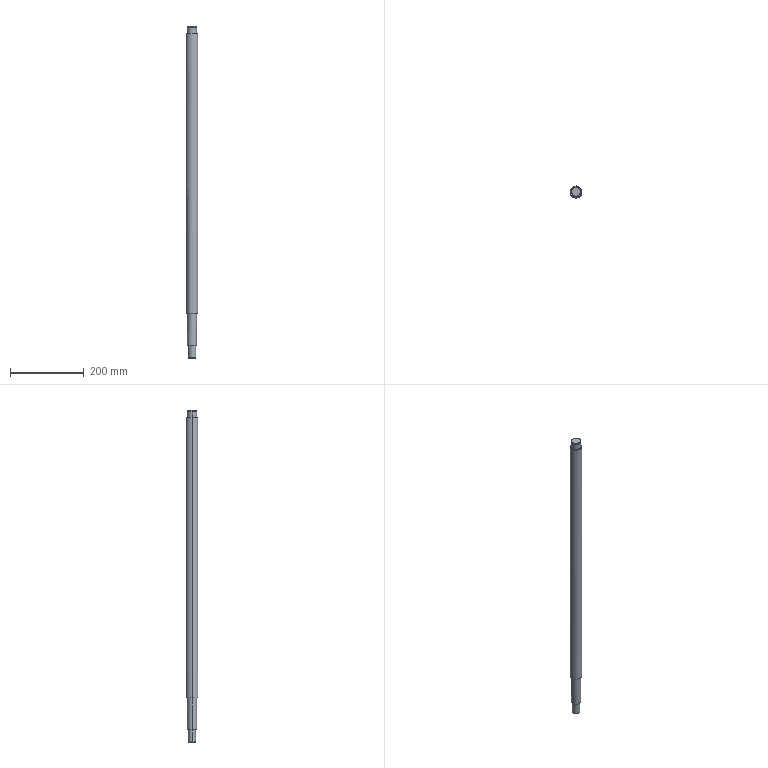Part | SolidWorks | features BaseBody 1 | 1 solid | 31 faces | box 32 x 32 x 900 mm | volume 673980 mm3 | cylinder 12 | cone 8 | plane 7 | spline 4 | commonest cylinder face diameters 25 x6 20 x2 23.9 x2 32 x2
STEP:
#1=CARTESIAN_POINT('',(-11.402,1598.781,-1156.3));
#2=VERTEX_POINT('',#1);
#3=CARTESIAN_POINT('',(-9.453,1592.079,-1156.3));
#4=VERTEX_POINT('',#3);
#5=CARTESIAN_POINT('',(-21.953,1592.079,-1156.3));
#6=DIRECTION('',(0.,0.,-1.));
#7=DIRECTION('',(-0.8441,-0.5362,0.));
#8=AXIS2_PLACEMENT_3D('',#5,#6,#7);
#9=CIRCLE('',#8,12.5);
#10=EDGE_CURVE('',#2,#4,#9,.T.);
#11=ORIENTED_EDGE('',*,*,#10,.F.);
#12=CARTESIAN_POINT('',(-11.149,1598.942,-1156.));
#13=VERTEX_POINT('',#12);
#14=CARTESIAN_POINT('',(-11.149,1598.942,-1156.3));
#15=DIRECTION('',(-0.5362,0.8441,0.));
#16=DIRECTION('',(0.8441,0.5362,0.));
#17=AXIS2_PLACEMENT_3D('',#14,#15,#16);
#18=CIRCLE('',#17,0.3);
#19=EDGE_CURVE('',#2,#13,#18,.T.);
#20=ORIENTED_EDGE('',*,*,#19,.T.);
#21=CARTESIAN_POINT('',(-32.758,1585.215,-1156.));
#22=VERTEX_POINT('',#21);
#23=CARTESIAN_POINT('',(-11.149,1598.942,-1156.));
#24=CARTESIAN_POINT('',(2.578,1577.333,-1156.));
#25=CARTESIAN_POINT('',(-19.031,1563.607,-1156.));
#26=CARTESIAN_POINT('',(-32.758,1585.215,-1156.));
#27=(BOUNDED_CURVE()B_SPLINE_CURVE(3,(#23,#24,#25,#26),.UNSPECIFIED.,.F.,.T.)B_SPLINE_CURVE_WITH_KNOTS((4,4),(0.,1.),.UNSPECIFIED.)CURVE()GEOMETRIC_REPRESENTATION_ITEM()RATIONAL_B_SPLINE_CURVE((1.,0.3333,0.3333,1.))REPRESENTATION_ITEM(''));
#28=EDGE_CURVE('',#13,#22,#27,.T.);
#29=ORIENTED_EDGE('',*,*,#28,.T.);
#30=CARTESIAN_POINT('',(-32.505,1585.376,-1156.3));
#31=VERTEX_POINT('',#30);
#32=CARTESIAN_POINT('',(-32.758,1585.215,-1156.3));
#33=DIRECTION('',(0.5362,-0.8441,0.));
#34=DIRECTION('',(-0.8441,-0.5362,0.));
#35=AXIS2_PLACEMENT_3D('',#32,#33,#34);
#36=CIRCLE('',#35,0.3);
#37=EDGE_CURVE('',#31,#22,#36,.T.);
#38=ORIENTED_EDGE('',*,*,#37,.F.);
#39=CARTESIAN_POINT('',(-21.953,1592.079,-1156.3));
#40=DIRECTION('',(0.,0.,-1.));
#41=DIRECTION('',(-0.8441,-0.5362,0.));
#42=AXIS2_PLACEMENT_3D('',#39,#40,#41);
#43=CIRCLE('',#42,12.5);
#44=EDGE_CURVE('',#4,#31,#43,.T.);
#45=ORIENTED_EDGE('',*,*,#44,.F.);
#46=EDGE_LOOP('',(#11,#20,#29,#38,#45));
#47=FACE_OUTER_BOUND('',#46,.T.);
#48=CARTESIAN_POINT('',(-32.505,1585.376,-1156.3));
#49=CARTESIAN_POINT('',(-19.099,1564.274,-1156.3));
#50=CARTESIAN_POINT('',(2.003,1577.679,-1156.3));
#51=CARTESIAN_POINT('',(-11.402,1598.781,-1156.3));
#52=CARTESIAN_POINT('',(-32.505,1585.376,-1156.124));
#53=CARTESIAN_POINT('',(-19.099,1564.274,-1156.124));
#54=CARTESIAN_POINT('',(2.003,1577.679,-1156.124));
#55=CARTESIAN_POINT('',(-11.402,1598.781,-1156.124));
#56=CARTESIAN_POINT('',(-32.609,1585.309,-1156.));
#57=CARTESIAN_POINT('',(-19.071,1563.997,-1156.));
#58=CARTESIAN_POINT('',(2.241,1577.536,-1156.));
#59=CARTESIAN_POINT('',(-11.298,1598.848,-1156.));
#60=CARTESIAN_POINT('',(-32.758,1585.215,-1156.));
#61=CARTESIAN_POINT('',(-19.031,1563.607,-1156.));
#62=CARTESIAN_POINT('',(2.578,1577.333,-1156.));
#63=CARTESIAN_POINT('',(-11.149,1598.942,-1156.));
#64=(BOUNDED_SURFACE()B_SPLINE_SURFACE(3,3,((#48,#49,#50,#51),(#52,#53,#54,#55),(#56,#57,#58,#59),(#60,#61,#62,#63)),.UNSPECIFIED.,.F.,.F.,.F.)B_SPLINE_SURFACE_WITH_KNOTS((4,4),(4,4),(0.,1.),(0.,1.),.UNSPECIFIED.)GEOMETRIC_REPRESENTATION_ITEM()RATIONAL_B_SPLINE_SURFACE(((1.,0.3333,0.3333,1.),(0.8047,0.2682,0.2682,0.8047),(0.8047,0.2682,0.2682,0.8047),(1.,0.3333,0.3333,1.)))REPRESENTATION_ITEM('')SURFACE());
#65=ADVANCED_FACE('',(#47),#64,.F.);
#66=CARTESIAN_POINT('',(-32.758,1585.215,-396.));
#67=VERTEX_POINT('',#66);
#68=CARTESIAN_POINT('',(-11.149,1598.942,-396.));
#69=VERTEX_POINT('',#68);
#70=CARTESIAN_POINT('',(-32.758,1585.215,-396.));
#71=CARTESIAN_POINT('',(-19.031,1563.607,-396.));
#72=CARTESIAN_POINT('',(2.578,1577.333,-396.));
#73=CARTESIAN_POINT('',(-11.149,1598.942,-396.));
#74=(BOUNDED_CURVE()B_SPLINE_CURVE(3,(#70,#71,#72,#73),.UNSPECIFIED.,.F.,.T.)B_SPLINE_CURVE_WITH_KNOTS((4,4),(0.,1.),.UNSPECIFIED.)CURVE()GEOMETRIC_REPRESENTATION_ITEM()RATIONAL_B_SPLINE_CURVE((1.,0.3333,0.3333,1.))REPRESENTATION_ITEM(''));
#75=EDGE_CURVE('',#67,#69,#74,.T.);
#76=ORIENTED_EDGE('',*,*,#75,.T.);
#77=CARTESIAN_POINT('',(-11.402,1598.781,-395.7));
#78=VERTEX_POINT('',#77);
#79=CARTESIAN_POINT('',(-11.149,1598.942,-395.7));
#80=DIRECTION('',(-0.5362,0.8441,0.));
#81=DIRECTION('',(0.8441,0.5362,0.));
#82=AXIS2_PLACEMENT_3D('',#79,#80,#81);
#83=CIRCLE('',#82,0.3);
#84=EDGE_CURVE('',#69,#78,#83,.T.);
#85=ORIENTED_EDGE('',*,*,#84,.T.);
#86=CARTESIAN_POINT('',(-9.453,1592.079,-395.7));
#87=VERTEX_POINT('',#86);
#88=CARTESIAN_POINT('',(-21.953,1592.079,-395.7));
#89=DIRECTION('',(0.,0.,1.));
#90=DIRECTION('',(-0.8441,-0.5362,0.));
#91=AXIS2_PLACEMENT_3D('',#88,#89,#90);
#92=CIRCLE('',#91,12.5);
#93=EDGE_CURVE('',#87,#78,#92,.T.);
#94=ORIENTED_EDGE('',*,*,#93,.F.);
#95=CARTESIAN_POINT('',(-32.505,1585.376,-395.7));
#96=VERTEX_POINT('',#95);
#97=CARTESIAN_POINT('',(-21.953,1592.079,-395.7));
#98=DIRECTION('',(0.,0.,1.));
#99=DIRECTION('',(-0.8441,-0.5362,0.));
#100=AXIS2_PLACEMENT_3D('',#97,#98,#99);
#101=CIRCLE('',#100,12.5);
#102=EDGE_CURVE('',#96,#87,#101,.T.);
#103=ORIENTED_EDGE('',*,*,#102,.F.);
#104=CARTESIAN_POINT('',(-32.758,1585.215,-395.7));
#105=DIRECTION('',(0.5362,-0.8441,0.));
#106=DIRECTION('',(-0.8441,-0.5362,0.));
#107=AXIS2_PLACEMENT_3D('',#104,#105,#106);
#108=CIRCLE('',#107,0.3);
#109=EDGE_CURVE('',#67,#96,#108,.T.);
#110=ORIENTED_EDGE('',*,*,#109,.F.);
#111=EDGE_LOOP('',(#76,#85,#94,#103,#110));
#112=FACE_OUTER_BOUND('',#111,.T.);
#113=CARTESIAN_POINT('',(-32.758,1585.215,-396.));
#114=CARTESIAN_POINT('',(-19.031,1563.607,-396.));
#115=CARTESIAN_POINT('',(2.578,1577.333,-396.));
#116=CARTESIAN_POINT('',(-11.149,1598.942,-396.));
#117=CARTESIAN_POINT('',(-32.609,1585.309,-396.));
#118=CARTESIAN_POINT('',(-19.071,1563.997,-396.));
#119=CARTESIAN_POINT('',(2.241,1577.536,-396.));
#120=CARTESIAN_POINT('',(-11.298,1598.848,-396.));
#121=CARTESIAN_POINT('',(-32.505,1585.376,-395.876));
#122=CARTESIAN_POINT('',(-19.099,1564.274,-395.876));
#123=CARTESIAN_POINT('',(2.003,1577.679,-395.876));
#124=CARTESIAN_POINT('',(-11.402,1598.781,-395.876));
#125=CARTESIAN_POINT('',(-32.505,1585.376,-395.7));
#126=CARTESIAN_POINT('',(-19.099,1564.274,-395.7));
#127=CARTESIAN_POINT('',(2.003,1577.679,-395.7));
#128=CARTESIAN_POINT('',(-11.402,1598.781,-395.7));
#129=(BOUNDED_SURFACE()B_SPLINE_SURFACE(3,3,((#113,#114,#115,#116),(#117,#118,#119,#120),(#121,#122,#123,#124),(#125,#126,#127,#128)),.UNSPECIFIED.,.F.,.F.,.F.)B_SPLINE_SURFACE_WITH_KNOTS((4,4),(4,4),(0.,1.),(0.,1.),.UNSPECIFIED.)GEOMETRIC_REPRESENTATION_ITEM()RATIONAL_B_SPLINE_SURFACE(((1.,0.3333,0.3333,1.),(0.8047,0.2682,0.2682,0.8047),(0.8047,0.2682,0.2682,0.8047),(1.,0.3333,0.3333,1.)))REPRESENTATION_ITEM('')SURFACE());
#130=ADVANCED_FACE('',(#112),#129,.F.);
#131=CARTESIAN_POINT('',(-5.953,1592.079,-1156.));
#132=VERTEX_POINT('',#131);
#133=CARTESIAN_POINT('',(-37.953,1592.079,-1156.));
#134=VERTEX_POINT('',#133);
#135=CARTESIAN_POINT('',(-21.953,1592.079,-1156.));
#136=DIRECTION('',(0.,0.,1.));
#137=DIRECTION('',(1.,0.,0.));
#138=AXIS2_PLACEMENT_3D('',#135,#136,#137);
#139=CIRCLE('',#138,16.);
#140=EDGE_CURVE('',#132,#134,#139,.T.);
#141=ORIENTED_EDGE('',*,*,#140,.T.);
#142=CARTESIAN_POINT('',(-37.953,1592.079,-396.5));
#143=VERTEX_POINT('',#142);
#144=CARTESIAN_POINT('',(-37.953,1592.079,-1276.));
#145=DIRECTION('',(0.,0.,1.));
#146=VECTOR('',#145,1000.);
#147=LINE('',#144,#146);
#148=EDGE_CURVE('',#134,#143,#147,.T.);
#149=ORIENTED_EDGE('',*,*,#148,.T.);
#150=CARTESIAN_POINT('',(-21.953,1608.079,-396.5));
#151=VERTEX_POINT('',#150);
#152=CARTESIAN_POINT('',(-21.953,1592.079,-396.5));
#153=DIRECTION('',(0.,0.,-1.));
#154=DIRECTION('',(1.,0.,0.));
#155=AXIS2_PLACEMENT_3D('',#152,#153,#154);
#156=CIRCLE('',#155,16.);
#157=EDGE_CURVE('',#143,#151,#156,.T.);
#158=ORIENTED_EDGE('',*,*,#157,.T.);
#159=CARTESIAN_POINT('',(-5.953,1592.079,-396.5));
#160=VERTEX_POINT('',#159);
#161=CARTESIAN_POINT('',(-21.953,1592.079,-396.5));
#162=DIRECTION('',(0.,0.,-1.));
#163=DIRECTION('',(1.,0.,0.));
#164=AXIS2_PLACEMENT_3D('',#161,#162,#163);
#165=CIRCLE('',#164,16.);
#166=EDGE_CURVE('',#151,#160,#165,.T.);
#167=ORIENTED_EDGE('',*,*,#166,.T.);
#168=CARTESIAN_POINT('',(-5.953,1592.079,-1276.));
#169=DIRECTION('',(0.,0.,1.));
#170=VECTOR('',#169,1000.);
#171=LINE('',#168,#170);
#172=EDGE_CURVE('',#132,#160,#171,.T.);
#173=ORIENTED_EDGE('',*,*,#172,.F.);
#174=EDGE_LOOP('',(#141,#149,#158,#167,#173));
#175=FACE_OUTER_BOUND('',#174,.T.);
#176=CARTESIAN_POINT('',(-21.953,1592.079,-1276.));
#177=DIRECTION('',(0.,0.,1.));
#178=DIRECTION('',(1.,0.,0.));
#179=AXIS2_PLACEMENT_3D('',#176,#177,#178);
#180=CYLINDRICAL_SURFACE('',#179,16.);
#181=ADVANCED_FACE('',(#175),#180,.T.);
#182=CARTESIAN_POINT('',(-21.953,1607.579,-396.));
#183=VERTEX_POINT('',#182);
#184=CARTESIAN_POINT('',(-21.953,1576.579,-396.));
#185=VERTEX_POINT('',#184);
#186=CARTESIAN_POINT('',(-21.953,1592.079,-396.));
#187=DIRECTION('',(0.,0.,-1.));
#188=DIRECTION('',(0.,1.,0.));
#189=AXIS2_PLACEMENT_3D('',#186,#187,#188);
#190=CIRCLE('',#189,15.5);
#191=EDGE_CURVE('',#183,#185,#190,.T.);
#192=ORIENTED_EDGE('',*,*,#191,.T.);
#193=CARTESIAN_POINT('',(-21.953,1576.079,-396.5));
#194=VERTEX_POINT('',#193);
#195=CARTESIAN_POINT('',(-21.953,1576.079,-396.5));
#196=DIRECTION('',(0.,-0.7071,-0.7071));
#197=VECTOR('',#196,1000.);
#198=LINE('',#195,#197);
#199=EDGE_CURVE('',#185,#194,#198,.T.);
#200=ORIENTED_EDGE('',*,*,#199,.T.);
#201=CARTESIAN_POINT('',(-21.953,1592.079,-396.5));
#202=DIRECTION('',(0.,0.,-1.));
#203=DIRECTION('',(1.,0.,0.));
#204=AXIS2_PLACEMENT_3D('',#201,#202,#203);
#205=CIRCLE('',#204,16.);
#206=EDGE_CURVE('',#160,#194,#205,.T.);
#207=ORIENTED_EDGE('',*,*,#206,.F.);
#208=ORIENTED_EDGE('',*,*,#166,.F.);
#209=CARTESIAN_POINT('',(-21.953,1608.079,-396.5));
#210=DIRECTION('',(0.,0.7071,-0.7071));
#211=VECTOR('',#210,1000.);
#212=LINE('',#209,#211);
#213=EDGE_CURVE('',#183,#151,#212,.T.);
#214=ORIENTED_EDGE('',*,*,#213,.F.);
#215=EDGE_LOOP('',(#192,#200,#207,#208,#214));
#216=FACE_OUTER_BOUND('',#215,.T.);
#217=CARTESIAN_POINT('',(-21.953,1592.079,-396.5));
#218=DIRECTION('',(0.,0.,-1.));
#219=DIRECTION('',(0.,1.,0.));
#220=AXIS2_PLACEMENT_3D('',#217,#218,#219);
#221=CONICAL_SURFACE('',#220,16.,0.7854);
#222=ADVANCED_FACE('',(#216),#221,.T.);
#223=CARTESIAN_POINT('',(-9.453,1592.079,-1242.5));
#224=VERTEX_POINT('',#223);
#225=CARTESIAN_POINT('',(-34.453,1592.079,-1242.5));
#226=VERTEX_POINT('',#225);
#227=CARTESIAN_POINT('',(-21.953,1592.079,-1242.5));
#228=DIRECTION('',(0.,0.,1.));
#229=DIRECTION('',(1.,0.,0.));
#230=AXIS2_PLACEMENT_3D('',#227,#228,#229);
#231=CIRCLE('',#230,12.5);
#232=EDGE_CURVE('',#224,#226,#231,.T.);
#233=ORIENTED_EDGE('',*,*,#232,.T.);
#234=CARTESIAN_POINT('',(-34.453,1592.079,-1156.3));
#235=VERTEX_POINT('',#234);
#236=CARTESIAN_POINT('',(-34.453,1592.079,-1276.));
#237=DIRECTION('',(0.,0.,1.));
#238=VECTOR('',#237,1000.);
#239=LINE('',#236,#238);
#240=EDGE_CURVE('',#226,#235,#239,.T.);
#241=ORIENTED_EDGE('',*,*,#240,.T.);
#242=CARTESIAN_POINT('',(-21.953,1592.079,-1156.3));
#243=DIRECTION('',(0.,0.,-1.));
#244=DIRECTION('',(-0.8441,-0.5362,0.));
#245=AXIS2_PLACEMENT_3D('',#242,#243,#244);
#246=CIRCLE('',#245,12.5);
#247=EDGE_CURVE('',#235,#2,#246,.T.);
#248=ORIENTED_EDGE('',*,*,#247,.T.);
#249=ORIENTED_EDGE('',*,*,#10,.T.);
#250=CARTESIAN_POINT('',(-9.453,1592.079,-1276.));
#251=DIRECTION('',(0.,0.,1.));
#252=VECTOR('',#251,1000.);
#253=LINE('',#250,#252);
#254=EDGE_CURVE('',#224,#4,#253,.T.);
#255=ORIENTED_EDGE('',*,*,#254,.F.);
#256=EDGE_LOOP('',(#233,#241,#248,#249,#255));
#257=FACE_OUTER_BOUND('',#256,.T.);
#258=CARTESIAN_POINT('',(-21.953,1592.079,-1276.));
#259=DIRECTION('',(0.,0.,1.));
#260=DIRECTION('',(1.,0.,0.));
#261=AXIS2_PLACEMENT_3D('',#258,#259,#260);
#262=CYLINDRICAL_SURFACE('',#261,12.5);
#263=ADVANCED_FACE('',(#257),#262,.T.);
#264=ORIENTED_EDGE('',*,*,#93,.T.);
#265=CARTESIAN_POINT('',(-34.453,1592.079,-395.7));
#266=VERTEX_POINT('',#265);
#267=CARTESIAN_POINT('',(-21.953,1592.079,-395.7));
#268=DIRECTION('',(0.,0.,1.));
#269=DIRECTION('',(-0.8441,-0.5362,0.));
#270=AXIS2_PLACEMENT_3D('',#267,#268,#269);
#271=CIRCLE('',#270,12.5);
#272=EDGE_CURVE('',#78,#266,#271,.T.);
#273=ORIENTED_EDGE('',*,*,#272,.T.);
#274=CARTESIAN_POINT('',(-34.453,1592.079,-381.));
#275=VERTEX_POINT('',#274);
#276=CARTESIAN_POINT('',(-34.453,1592.079,-396.));
#277=DIRECTION('',(0.,0.,1.));
#278=VECTOR('',#277,1000.);
#279=LINE('',#276,#278);
#280=EDGE_CURVE('',#266,#275,#279,.T.);
#281=ORIENTED_EDGE('',*,*,#280,.T.);
#282=CARTESIAN_POINT('',(-9.453,1592.079,-381.));
#283=VERTEX_POINT('',#282);
#284=CARTESIAN_POINT('',(-21.953,1592.079,-381.));
#285=DIRECTION('',(0.,0.,-1.));
#286=DIRECTION('',(1.,0.,0.));
#287=AXIS2_PLACEMENT_3D('',#284,#285,#286);
#288=CIRCLE('',#287,12.5);
#289=EDGE_CURVE('',#275,#283,#288,.T.);
#290=ORIENTED_EDGE('',*,*,#289,.T.);
#291=CARTESIAN_POINT('',(-9.453,1592.079,-396.));
#292=DIRECTION('',(0.,0.,1.));
#293=VECTOR('',#292,1000.);
#294=LINE('',#291,#293);
#295=EDGE_CURVE('',#87,#283,#294,.T.);
#296=ORIENTED_EDGE('',*,*,#295,.F.);
#297=EDGE_LOOP('',(#264,#273,#281,#290,#296));
#298=FACE_OUTER_BOUND('',#297,.T.);
#299=CARTESIAN_POINT('',(-21.953,1592.079,-396.));
#300=DIRECTION('',(0.,0.,1.));
#301=DIRECTION('',(1.,0.,0.));
#302=AXIS2_PLACEMENT_3D('',#299,#300,#301);
#303=CYLINDRICAL_SURFACE('',#302,12.5);
#304=ADVANCED_FACE('',(#298),#303,.T.);
#305=CARTESIAN_POINT('',(-9.953,1592.079,-1243.));
#306=VERTEX_POINT('',#305);
#307=CARTESIAN_POINT('',(-33.953,1592.079,-1243.));
#308=VERTEX_POINT('',#307);
#309=CARTESIAN_POINT('',(-21.953,1592.079,-1243.));
#310=DIRECTION('',(0.,0.,1.));
#311=DIRECTION('',(1.,0.,0.));
#312=AXIS2_PLACEMENT_3D('',#309,#310,#311);
#313=CIRCLE('',#312,12.);
#314=EDGE_CURVE('',#306,#308,#313,.T.);
#315=ORIENTED_EDGE('',*,*,#314,.T.);
#316=CARTESIAN_POINT('',(-34.453,1592.079,-1242.5));
#317=DIRECTION('',(-0.7071,0.,0.7071));
#318=VECTOR('',#317,1000.);
#319=LINE('',#316,#318);
#320=EDGE_CURVE('',#308,#226,#319,.T.);
#321=ORIENTED_EDGE('',*,*,#320,.T.);
#322=ORIENTED_EDGE('',*,*,#232,.F.);
#323=CARTESIAN_POINT('',(-9.453,1592.079,-1242.5));
#324=DIRECTION('',(0.7071,0.,0.7071));
#325=VECTOR('',#324,1000.);
#326=LINE('',#323,#325);
#327=EDGE_CURVE('',#306,#224,#326,.T.);
#328=ORIENTED_EDGE('',*,*,#327,.F.);
#329=EDGE_LOOP('',(#315,#321,#322,#328));
#330=FACE_OUTER_BOUND('',#329,.T.);
#331=CARTESIAN_POINT('',(-21.953,1592.079,-1242.5));
#332=DIRECTION('',(0.,0.,1.));
#333=DIRECTION('',(1.,0.,0.));
#334=AXIS2_PLACEMENT_3D('',#331,#332,#333);
#335=CONICAL_SURFACE('',#334,12.5,0.7854);
#336=ADVANCED_FACE('',(#330),#335,.T.);
#337=CARTESIAN_POINT('',(-10.003,1592.079,-381.));
#338=VERTEX_POINT('',#337);
#339=CARTESIAN_POINT('',(-33.903,1592.079,-381.));
#340=VERTEX_POINT('',#339);
#341=CARTESIAN_POINT('',(-21.953,1592.079,-381.));
#342=DIRECTION('',(0.,0.,1.));
#343=DIRECTION('',(1.,0.,0.));
#344=AXIS2_PLACEMENT_3D('',#341,#342,#343);
#345=CIRCLE('',#344,11.95);
#346=EDGE_CURVE('',#338,#340,#345,.T.);
#347=ORIENTED_EDGE('',*,*,#346,.T.);
#348=CARTESIAN_POINT('',(-33.903,1592.079,-379.65));
#349=VERTEX_POINT('',#348);
#350=CARTESIAN_POINT('',(-33.903,1592.079,-396.));
#351=DIRECTION('',(0.,0.,1.));
#352=VECTOR('',#351,1000.);
#353=LINE('',#350,#352);
#354=EDGE_CURVE('',#340,#349,#353,.T.);
#355=ORIENTED_EDGE('',*,*,#354,.T.);
#356=CARTESIAN_POINT('',(-10.003,1592.079,-379.65));
#357=VERTEX_POINT('',#356);
#358=CARTESIAN_POINT('',(-21.953,1592.079,-379.65));
#359=DIRECTION('',(0.,0.,-1.));
#360=DIRECTION('',(1.,0.,0.));
#361=AXIS2_PLACEMENT_3D('',#358,#359,#360);
#362=CIRCLE('',#361,11.95);
#363=EDGE_CURVE('',#349,#357,#362,.T.);
#364=ORIENTED_EDGE('',*,*,#363,.T.);
#365=CARTESIAN_POINT('',(-10.003,1592.079,-396.));
#366=DIRECTION('',(0.,0.,1.));
#367=VECTOR('',#366,1000.);
#368=LINE('',#365,#367);
#369=EDGE_CURVE('',#338,#357,#368,.T.);
#370=ORIENTED_EDGE('',*,*,#369,.F.);
#371=EDGE_LOOP('',(#347,#355,#364,#370));
#372=FACE_OUTER_BOUND('',#371,.T.);
#373=CARTESIAN_POINT('',(-21.953,1592.079,-396.));
#374=DIRECTION('',(0.,0.,1.));
#375=DIRECTION('',(1.,0.,0.));
#376=AXIS2_PLACEMENT_3D('',#373,#374,#375);
#377=CYLINDRICAL_SURFACE('',#376,11.95);
#378=ADVANCED_FACE('',(#372),#377,.T.);
#379=CARTESIAN_POINT('',(-11.953,1592.079,-1275.5));
#380=VERTEX_POINT('',#379);
#381=CARTESIAN_POINT('',(-31.953,1592.079,-1275.5));
#382=VERTEX_POINT('',#381);
#383=CARTESIAN_POINT('',(-21.953,1592.079,-1275.5));
#384=DIRECTION('',(0.,0.,1.));
#385=DIRECTION('',(1.,0.,0.));
#386=AXIS2_PLACEMENT_3D('',#383,#384,#385);
#387=CIRCLE('',#386,10.);
#388=EDGE_CURVE('',#380,#382,#387,.T.);
#389=ORIENTED_EDGE('',*,*,#388,.T.);
#390=CARTESIAN_POINT('',(-31.953,1592.079,-1243.));
#391=VERTEX_POINT('',#390);
#392=CARTESIAN_POINT('',(-31.953,1592.079,-1276.));
#393=DIRECTION('',(0.,0.,1.));
#394=VECTOR('',#393,1000.);
#395=LINE('',#392,#394);
#396=EDGE_CURVE('',#382,#391,#395,.T.);
#397=ORIENTED_EDGE('',*,*,#396,.T.);
#398=CARTESIAN_POINT('',(-11.953,1592.079,-1243.));
#399=VERTEX_POINT('',#398);
#400=CARTESIAN_POINT('',(-21.953,1592.079,-1243.));
#401=DIRECTION('',(0.,0.,-1.));
#402=DIRECTION('',(1.,0.,0.));
#403=AXIS2_PLACEMENT_3D('',#400,#401,#402);
#404=CIRCLE('',#403,10.);
#405=EDGE_CURVE('',#391,#399,#404,.T.);
#406=ORIENTED_EDGE('',*,*,#405,.T.);
#407=CARTESIAN_POINT('',(-11.953,1592.079,-1276.));
#408=DIRECTION('',(0.,0.,1.));
#409=VECTOR('',#408,1000.);
#410=LINE('',#407,#409);
#411=EDGE_CURVE('',#380,#399,#410,.T.);
#412=ORIENTED_EDGE('',*,*,#411,.F.);
#413=EDGE_LOOP('',(#389,#397,#406,#412));
#414=FACE_OUTER_BOUND('',#413,.T.);
#415=CARTESIAN_POINT('',(-21.953,1592.079,-1276.));
#416=DIRECTION('',(0.,0.,1.));
#417=DIRECTION('',(1.,0.,0.));
#418=AXIS2_PLACEMENT_3D('',#415,#416,#417);
#419=CYLINDRICAL_SURFACE('',#418,10.);
#420=ADVANCED_FACE('',(#414),#419,.T.);
#421=CARTESIAN_POINT('',(-12.453,1592.079,-1276.));
#422=VERTEX_POINT('',#421);
#423=CARTESIAN_POINT('',(-31.453,1592.079,-1276.));
#424=VERTEX_POINT('',#423);
#425=CARTESIAN_POINT('',(-21.953,1592.079,-1276.));
#426=DIRECTION('',(0.,0.,1.));
#427=DIRECTION('',(1.,0.,0.));
#428=AXIS2_PLACEMENT_3D('',#425,#426,#427);
#429=CIRCLE('',#428,9.5);
#430=EDGE_CURVE('',#422,#424,#429,.T.);
#431=ORIENTED_EDGE('',*,*,#430,.T.);
#432=CARTESIAN_POINT('',(-31.953,1592.079,-1275.5));
#433=DIRECTION('',(-0.7071,0.,0.7071));
#434=VECTOR('',#433,1000.);
#435=LINE('',#432,#434);
#436=EDGE_CURVE('',#424,#382,#435,.T.);
#437=ORIENTED_EDGE('',*,*,#436,.T.);
#438=ORIENTED_EDGE('',*,*,#388,.F.);
#439=CARTESIAN_POINT('',(-11.953,1592.079,-1275.5));
#440=DIRECTION('',(0.7071,0.,0.7071));
#441=VECTOR('',#440,1000.);
#442=LINE('',#439,#441);
#443=EDGE_CURVE('',#422,#380,#442,.T.);
#444=ORIENTED_EDGE('',*,*,#443,.F.);
#445=EDGE_LOOP('',(#431,#437,#438,#444));
#446=FACE_OUTER_BOUND('',#445,.T.);
#447=CARTESIAN_POINT('',(-21.953,1592.079,-1275.5));
#448=DIRECTION('',(0.,0.,1.));
#449=DIRECTION('',(1.,0.,0.));
#450=AXIS2_PLACEMENT_3D('',#447,#448,#449);
#451=CONICAL_SURFACE('',#450,10.,0.7854);
#452=ADVANCED_FACE('',(#446),#451,.T.);
#453=CARTESIAN_POINT('',(-9.453,1592.079,-379.65));
#454=VERTEX_POINT('',#453);
#455=CARTESIAN_POINT('',(-34.453,1592.079,-379.65));
#456=VERTEX_POINT('',#455);
#457=CARTESIAN_POINT('',(-21.953,1592.079,-379.65));
#458=DIRECTION('',(0.,0.,1.));
#459=DIRECTION('',(1.,0.,0.));
#460=AXIS2_PLACEMENT_3D('',#457,#458,#459);
#461=CIRCLE('',#460,12.5);
#462=EDGE_CURVE('',#454,#456,#461,.T.);
#463=ORIENTED_EDGE('',*,*,#462,.T.);
#464=CARTESIAN_POINT('',(-34.453,1592.079,-376.5));
#465=VERTEX_POINT('',#464);
#466=CARTESIAN_POINT('',(-34.453,1592.079,-396.));
#467=DIRECTION('',(0.,0.,1.));
#468=VECTOR('',#467,1000.);
#469=LINE('',#466,#468);
#470=EDGE_CURVE('',#456,#465,#469,.T.);
#471=ORIENTED_EDGE('',*,*,#470,.T.);
#472=CARTESIAN_POINT('',(-9.453,1592.079,-376.5));
#473=VERTEX_POINT('',#472);
#474=CARTESIAN_POINT('',(-21.953,1592.079,-376.5));
#475=DIRECTION('',(0.,0.,-1.));
#476=DIRECTION('',(1.,0.,0.));
#477=AXIS2_PLACEMENT_3D('',#474,#475,#476);
#478=CIRCLE('',#477,12.5);
#479=EDGE_CURVE('',#465,#473,#478,.T.);
#480=ORIENTED_EDGE('',*,*,#479,.T.);
#481=CARTESIAN_POINT('',(-9.453,1592.079,-396.));
#482=DIRECTION('',(0.,0.,1.));
#483=VECTOR('',#482,1000.);
#484=LINE('',#481,#483);
#485=EDGE_CURVE('',#454,#473,#484,.T.);
#486=ORIENTED_EDGE('',*,*,#485,.F.);
#487=EDGE_LOOP('',(#463,#471,#480,#486));
#488=FACE_OUTER_BOUND('',#487,.T.);
#489=CARTESIAN_POINT('',(-21.953,1592.079,-396.));
#490=DIRECTION('',(0.,0.,1.));
#491=DIRECTION('',(1.,0.,0.));
#492=AXIS2_PLACEMENT_3D('',#489,#490,#491);
#493=CYLINDRICAL_SURFACE('',#492,12.5);
#494=ADVANCED_FACE('',(#488),#493,.T.);
#495=CARTESIAN_POINT('',(-33.953,1592.079,-376.));
#496=VERTEX_POINT('',#495);
#497=CARTESIAN_POINT('',(-9.953,1592.079,-376.));
#498=VERTEX_POINT('',#497);
#499=CARTESIAN_POINT('',(-21.953,1592.079,-376.));
#500=DIRECTION('',(0.,0.,-1.));
#501=DIRECTION('',(-1.,0.,0.));
#502=AXIS2_PLACEMENT_3D('',#499,#500,#501);
#503=CIRCLE('',#502,12.);
#504=EDGE_CURVE('',#496,#498,#503,.T.);
#505=ORIENTED_EDGE('',*,*,#504,.T.);
#506=CARTESIAN_POINT('',(-9.453,1592.079,-376.5));
#507=DIRECTION('',(0.7071,0.,-0.7071));
#508=VECTOR('',#507,1000.);
#509=LINE('',#506,#508);
#510=EDGE_CURVE('',#498,#473,#509,.T.);
#511=ORIENTED_EDGE('',*,*,#510,.T.);
#512=ORIENTED_EDGE('',*,*,#479,.F.);
#513=CARTESIAN_POINT('',(-34.453,1592.079,-376.5));
#514=DIRECTION('',(-0.7071,0.,-0.7071));
#515=VECTOR('',#514,1000.);
#516=LINE('',#513,#515);
#517=EDGE_CURVE('',#496,#465,#516,.T.);
#518=ORIENTED_EDGE('',*,*,#517,.F.);
#519=EDGE_LOOP('',(#505,#511,#512,#518));
#520=FACE_OUTER_BOUND('',#519,.T.);
#521=CARTESIAN_POINT('',(-21.953,1592.079,-376.5));
#522=DIRECTION('',(0.,0.,-1.));
#523=DIRECTION('',(-1.,0.,0.));
#524=AXIS2_PLACEMENT_3D('',#521,#522,#523);
#525=CONICAL_SURFACE('',#524,12.5,0.7854);
#526=ADVANCED_FACE('',(#520),#525,.T.);
#527=ORIENTED_EDGE('',*,*,#148,.F.);
#528=CARTESIAN_POINT('',(-21.953,1592.079,-1156.));
#529=DIRECTION('',(0.,0.,1.));
#530=DIRECTION('',(1.,0.,0.));
#531=AXIS2_PLACEMENT_3D('',#528,#529,#530);
#532=CIRCLE('',#531,16.);
#533=EDGE_CURVE('',#134,#132,#532,.T.);
#534=ORIENTED_EDGE('',*,*,#533,.T.);
#535=ORIENTED_EDGE('',*,*,#172,.T.);
#536=ORIENTED_EDGE('',*,*,#206,.T.);
#537=CARTESIAN_POINT('',(-21.953,1592.079,-396.5));
#538=DIRECTION('',(0.,0.,-1.));
#539=DIRECTION('',(1.,0.,0.));
#540=AXIS2_PLACEMENT_3D('',#537,#538,#539);
#541=CIRCLE('',#540,16.);
#542=EDGE_CURVE('',#194,#143,#541,.T.);
#543=ORIENTED_EDGE('',*,*,#542,.T.);
#544=EDGE_LOOP('',(#527,#534,#535,#536,#543));
#545=FACE_OUTER_BOUND('',#544,.T.);
#546=CARTESIAN_POINT('',(-21.953,1592.079,-1276.));
#547=DIRECTION('',(0.,0.,1.));
#548=DIRECTION('',(1.,0.,0.));
#549=AXIS2_PLACEMENT_3D('',#546,#547,#548);
#550=CYLINDRICAL_SURFACE('',#549,16.);
#551=ADVANCED_FACE('',(#545),#550,.T.);
#552=ORIENTED_EDGE('',*,*,#199,.F.);
#553=CARTESIAN_POINT('',(-21.953,1592.079,-396.));
#554=DIRECTION('',(0.,0.,-1.));
#555=DIRECTION('',(0.,1.,0.));
#556=AXIS2_PLACEMENT_3D('',#553,#554,#555);
#557=CIRCLE('',#556,15.5);
#558=EDGE_CURVE('',#185,#183,#557,.T.);
#559=ORIENTED_EDGE('',*,*,#558,.T.);
#560=ORIENTED_EDGE('',*,*,#213,.T.);
#561=ORIENTED_EDGE('',*,*,#157,.F.);
#562=ORIENTED_EDGE('',*,*,#542,.F.);
#563=EDGE_LOOP('',(#552,#559,#560,#561,#562));
#564=FACE_OUTER_BOUND('',#563,.T.);
#565=CARTESIAN_POINT('',(-21.953,1592.079,-396.5));
#566=DIRECTION('',(0.,0.,-1.));
#567=DIRECTION('',(0.,1.,0.));
#568=AXIS2_PLACEMENT_3D('',#565,#566,#567);
#569=CONICAL_SURFACE('',#568,16.,0.7854);
#570=ADVANCED_FACE('',(#564),#569,.T.);
#571=ORIENTED_EDGE('',*,*,#28,.F.);
#572=CARTESIAN_POINT('',(-32.758,1585.215,-1156.));
#573=CARTESIAN_POINT('',(-36.778,1591.544,-1156.));
#574=CARTESIAN_POINT('',(-35.146,1598.862,-1156.));
#575=CARTESIAN_POINT('',(-28.817,1602.883,-1156.));
#576=CARTESIAN_POINT('',(-22.488,1606.903,-1156.));
#577=CARTESIAN_POINT('',(-15.17,1605.271,-1156.));
#578=CARTESIAN_POINT('',(-11.149,1598.942,-1156.));
#579=(BOUNDED_CURVE()B_SPLINE_CURVE(3,(#572,#573,#574,#575,#576,#577,#578),.UNSPECIFIED.,.F.,.T.)B_SPLINE_CURVE_WITH_KNOTS((4,3,4),(0.,0.5,1.),.UNSPECIFIED.)CURVE()GEOMETRIC_REPRESENTATION_ITEM()RATIONAL_B_SPLINE_CURVE((1.,0.8047,0.8047,1.,0.8047,0.8047,1.))REPRESENTATION_ITEM(''));
#580=EDGE_CURVE('',#22,#13,#579,.T.);
#581=ORIENTED_EDGE('',*,*,#580,.F.);
#582=EDGE_LOOP('',(#571,#581));
#583=FACE_BOUND('',#582,.T.);
#584=ORIENTED_EDGE('',*,*,#140,.F.);
#585=ORIENTED_EDGE('',*,*,#533,.F.);
#586=EDGE_LOOP('',(#584,#585));
#587=FACE_OUTER_BOUND('',#586,.T.);
#588=CARTESIAN_POINT('',(-13.374,1578.573,-1156.));
#589=DIRECTION('',(0.,0.,1.));
#590=DIRECTION('',(1.,0.,0.));
#591=AXIS2_PLACEMENT_3D('',#588,#589,#590);
#592=PLANE('',#591);
#593=ADVANCED_FACE('',(#583,#587),#592,.F.);
#594=CARTESIAN_POINT('',(-11.149,1598.942,-396.));
#595=CARTESIAN_POINT('',(-15.17,1605.271,-396.));
#596=CARTESIAN_POINT('',(-22.488,1606.903,-396.));
#597=CARTESIAN_POINT('',(-28.817,1602.883,-396.));
#598=CARTESIAN_POINT('',(-35.146,1598.862,-396.));
#599=CARTESIAN_POINT('',(-36.778,1591.544,-396.));
#600=CARTESIAN_POINT('',(-32.758,1585.215,-396.));
#601=(BOUNDED_CURVE()B_SPLINE_CURVE(3,(#594,#595,#596,#597,#598,#599,#600),.UNSPECIFIED.,.F.,.T.)B_SPLINE_CURVE_WITH_KNOTS((4,3,4),(0.,0.5,1.),.UNSPECIFIED.)CURVE()GEOMETRIC_REPRESENTATION_ITEM()RATIONAL_B_SPLINE_CURVE((1.,0.8047,0.8047,1.,0.8047,0.8047,1.))REPRESENTATION_ITEM(''));
#602=EDGE_CURVE('',#69,#67,#601,.T.);
#603=ORIENTED_EDGE('',*,*,#602,.F.);
#604=ORIENTED_EDGE('',*,*,#75,.F.);
#605=EDGE_LOOP('',(#603,#604));
#606=FACE_BOUND('',#605,.T.);
#607=ORIENTED_EDGE('',*,*,#191,.F.);
#608=ORIENTED_EDGE('',*,*,#558,.F.);
#609=EDGE_LOOP('',(#607,#608));
#610=FACE_OUTER_BOUND('',#609,.T.);
#611=CARTESIAN_POINT('',(-21.953,1592.079,-396.));
#612=DIRECTION('',(0.,0.,-1.));
#613=DIRECTION('',(-1.,0.,0.));
#614=AXIS2_PLACEMENT_3D('',#611,#612,#613);
#615=PLANE('',#614);
#616=ADVANCED_FACE('',(#606,#610),#615,.F.);
#617=ORIENTED_EDGE('',*,*,#19,.F.);
#618=ORIENTED_EDGE('',*,*,#247,.F.);
#619=CARTESIAN_POINT('',(-21.953,1592.079,-1156.3));
#620=DIRECTION('',(0.,0.,-1.));
#621=DIRECTION('',(-0.8441,-0.5362,0.));
#622=AXIS2_PLACEMENT_3D('',#619,#620,#621);
#623=CIRCLE('',#622,12.5);
#624=EDGE_CURVE('',#31,#235,#623,.T.);
#625=ORIENTED_EDGE('',*,*,#624,.F.);
#626=ORIENTED_EDGE('',*,*,#37,.T.);
#627=ORIENTED_EDGE('',*,*,#580,.T.);
#628=EDGE_LOOP('',(#617,#618,#625,#626,#627));
#629=FACE_OUTER_BOUND('',#628,.T.);
#630=CARTESIAN_POINT('',(-11.402,1598.781,-1156.3));
#631=CARTESIAN_POINT('',(-15.329,1604.962,-1156.3));
#632=CARTESIAN_POINT('',(-22.475,1606.556,-1156.3));
#633=CARTESIAN_POINT('',(-28.656,1602.63,-1156.3));
#634=CARTESIAN_POINT('',(-34.837,1598.703,-1156.3));
#635=CARTESIAN_POINT('',(-36.431,1591.557,-1156.3));
#636=CARTESIAN_POINT('',(-32.505,1585.376,-1156.3));
#637=CARTESIAN_POINT('',(-11.402,1598.781,-1156.124));
#638=CARTESIAN_POINT('',(-15.329,1604.962,-1156.124));
#639=CARTESIAN_POINT('',(-22.475,1606.556,-1156.124));
#640=CARTESIAN_POINT('',(-28.656,1602.63,-1156.124));
#641=CARTESIAN_POINT('',(-34.837,1598.703,-1156.124));
#642=CARTESIAN_POINT('',(-36.431,1591.557,-1156.124));
#643=CARTESIAN_POINT('',(-32.505,1585.376,-1156.124));
#644=CARTESIAN_POINT('',(-11.298,1598.848,-1156.));
#645=CARTESIAN_POINT('',(-15.263,1605.09,-1156.));
#646=CARTESIAN_POINT('',(-22.481,1606.7,-1156.));
#647=CARTESIAN_POINT('',(-28.723,1602.735,-1156.));
#648=CARTESIAN_POINT('',(-34.965,1598.769,-1156.));
#649=CARTESIAN_POINT('',(-36.575,1591.551,-1156.));
#650=CARTESIAN_POINT('',(-32.609,1585.309,-1156.));
#651=CARTESIAN_POINT('',(-11.149,1598.942,-1156.));
#652=CARTESIAN_POINT('',(-15.17,1605.271,-1156.));
#653=CARTESIAN_POINT('',(-22.488,1606.903,-1156.));
#654=CARTESIAN_POINT('',(-28.817,1602.883,-1156.));
#655=CARTESIAN_POINT('',(-35.146,1598.862,-1156.));
#656=CARTESIAN_POINT('',(-36.778,1591.544,-1156.));
#657=CARTESIAN_POINT('',(-32.758,1585.215,-1156.));
#658=(BOUNDED_SURFACE()B_SPLINE_SURFACE(3,3,((#630,#631,#632,#633,#634,#635,#636),(#637,#638,#639,#640,#641,#642,#643),(#644,#645,#646,#647,#648,#649,#650),(#651,#652,#653,#654,#655,#656,#657)),.UNSPECIFIED.,.F.,.F.,.F.)B_SPLINE_SURFACE_WITH_KNOTS((4,4),(4,3,4),(0.,1.),(0.,0.5,1.),.UNSPECIFIED.)GEOMETRIC_REPRESENTATION_ITEM()RATIONAL_B_SPLINE_SURFACE(((1.,0.8047,0.8047,1.,0.8047,0.8047,1.),(0.8047,0.6476,0.6476,0.8047,0.6476,0.6476,0.8047),(0.8047,0.6476,0.6476,0.8047,0.6476,0.6476,0.8047),(1.,0.8047,0.8047,1.,0.8047,0.8047,1.)))REPRESENTATION_ITEM('')SURFACE());
#659=ADVANCED_FACE('',(#629),#658,.F.);
#660=ORIENTED_EDGE('',*,*,#84,.F.);
#661=ORIENTED_EDGE('',*,*,#602,.T.);
#662=ORIENTED_EDGE('',*,*,#109,.T.);
#663=CARTESIAN_POINT('',(-21.953,1592.079,-395.7));
#664=DIRECTION('',(0.,0.,1.));
#665=DIRECTION('',(-0.8441,-0.5362,0.));
#666=AXIS2_PLACEMENT_3D('',#663,#664,#665);
#667=CIRCLE('',#666,12.5);
#668=EDGE_CURVE('',#266,#96,#667,.T.);
#669=ORIENTED_EDGE('',*,*,#668,.F.);
#670=ORIENTED_EDGE('',*,*,#272,.F.);
#671=EDGE_LOOP('',(#660,#661,#662,#669,#670));
#672=FACE_OUTER_BOUND('',#671,.T.);
#673=CARTESIAN_POINT('',(-11.149,1598.942,-396.));
#674=CARTESIAN_POINT('',(-15.17,1605.271,-396.));
#675=CARTESIAN_POINT('',(-22.488,1606.903,-396.));
#676=CARTESIAN_POINT('',(-28.817,1602.883,-396.));
#677=CARTESIAN_POINT('',(-35.146,1598.862,-396.));
#678=CARTESIAN_POINT('',(-36.778,1591.544,-396.));
#679=CARTESIAN_POINT('',(-32.758,1585.215,-396.));
#680=CARTESIAN_POINT('',(-11.298,1598.848,-396.));
#681=CARTESIAN_POINT('',(-15.263,1605.09,-396.));
#682=CARTESIAN_POINT('',(-22.481,1606.7,-396.));
#683=CARTESIAN_POINT('',(-28.723,1602.735,-396.));
#684=CARTESIAN_POINT('',(-34.965,1598.769,-396.));
#685=CARTESIAN_POINT('',(-36.575,1591.551,-396.));
#686=CARTESIAN_POINT('',(-32.609,1585.309,-396.));
#687=CARTESIAN_POINT('',(-11.402,1598.781,-395.876));
#688=CARTESIAN_POINT('',(-15.329,1604.962,-395.876));
#689=CARTESIAN_POINT('',(-22.475,1606.556,-395.876));
#690=CARTESIAN_POINT('',(-28.656,1602.63,-395.876));
#691=CARTESIAN_POINT('',(-34.837,1598.703,-395.876));
#692=CARTESIAN_POINT('',(-36.431,1591.557,-395.876));
#693=CARTESIAN_POINT('',(-32.505,1585.376,-395.876));
#694=CARTESIAN_POINT('',(-11.402,1598.781,-395.7));
#695=CARTESIAN_POINT('',(-15.329,1604.962,-395.7));
#696=CARTESIAN_POINT('',(-22.475,1606.556,-395.7));
#697=CARTESIAN_POINT('',(-28.656,1602.63,-395.7));
#698=CARTESIAN_POINT('',(-34.837,1598.703,-395.7));
#699=CARTESIAN_POINT('',(-36.431,1591.557,-395.7));
#700=CARTESIAN_POINT('',(-32.505,1585.376,-395.7));
#701=(BOUNDED_SURFACE()B_SPLINE_SURFACE(3,3,((#673,#674,#675,#676,#677,#678,#679),(#680,#681,#682,#683,#684,#685,#686),(#687,#688,#689,#690,#691,#692,#693),(#694,#695,#696,#697,#698,#699,#700)),.UNSPECIFIED.,.F.,.F.,.F.)B_SPLINE_SURFACE_WITH_KNOTS((4,4),(4,3,4),(0.,1.),(0.,0.5,1.),.UNSPECIFIED.)GEOMETRIC_REPRESENTATION_ITEM()RATIONAL_B_SPLINE_SURFACE(((1.,0.8047,0.8047,1.,0.8047,0.8047,1.),(0.8047,0.6476,0.6476,0.8047,0.6476,0.6476,0.8047),(0.8047,0.6476,0.6476,0.8047,0.6476,0.6476,0.8047),(1.,0.8047,0.8047,1.,0.8047,0.8047,1.)))REPRESENTATION_ITEM('')SURFACE());
#702=ADVANCED_FACE('',(#672),#701,.F.);
#703=ORIENTED_EDGE('',*,*,#240,.F.);
#704=CARTESIAN_POINT('',(-21.953,1592.079,-1242.5));
#705=DIRECTION('',(0.,0.,1.));
#706=DIRECTION('',(1.,0.,0.));
#707=AXIS2_PLACEMENT_3D('',#704,#705,#706);
#708=CIRCLE('',#707,12.5);
#709=EDGE_CURVE('',#226,#224,#708,.T.);
#710=ORIENTED_EDGE('',*,*,#709,.T.);
#711=ORIENTED_EDGE('',*,*,#254,.T.);
#712=ORIENTED_EDGE('',*,*,#44,.T.);
#713=ORIENTED_EDGE('',*,*,#624,.T.);
#714=EDGE_LOOP('',(#703,#710,#711,#712,#713));
#715=FACE_OUTER_BOUND('',#714,.T.);
#716=CARTESIAN_POINT('',(-21.953,1592.079,-1276.));
#717=DIRECTION('',(0.,0.,1.));
#718=DIRECTION('',(1.,0.,0.));
#719=AXIS2_PLACEMENT_3D('',#716,#717,#718);
#720=CYLINDRICAL_SURFACE('',#719,12.5);
#721=ADVANCED_FACE('',(#715),#720,.T.);
#722=ORIENTED_EDGE('',*,*,#280,.F.);
#723=ORIENTED_EDGE('',*,*,#668,.T.);
#724=ORIENTED_EDGE('',*,*,#102,.T.);
#725=ORIENTED_EDGE('',*,*,#295,.T.);
#726=CARTESIAN_POINT('',(-21.953,1592.079,-381.));
#727=DIRECTION('',(0.,0.,-1.));
#728=DIRECTION('',(1.,0.,0.));
#729=AXIS2_PLACEMENT_3D('',#726,#727,#728);
#730=CIRCLE('',#729,12.5);
#731=EDGE_CURVE('',#283,#275,#730,.T.);
#732=ORIENTED_EDGE('',*,*,#731,.T.);
#733=EDGE_LOOP('',(#722,#723,#724,#725,#732));
#734=FACE_OUTER_BOUND('',#733,.T.);
#735=CARTESIAN_POINT('',(-21.953,1592.079,-396.));
#736=DIRECTION('',(0.,0.,1.));
#737=DIRECTION('',(1.,0.,0.));
#738=AXIS2_PLACEMENT_3D('',#735,#736,#737);
#739=CYLINDRICAL_SURFACE('',#738,12.5);
#740=ADVANCED_FACE('',(#734),#739,.T.);
#741=ORIENTED_EDGE('',*,*,#320,.F.);
#742=CARTESIAN_POINT('',(-21.953,1592.079,-1243.));
#743=DIRECTION('',(0.,0.,1.));
#744=DIRECTION('',(1.,0.,0.));
#745=AXIS2_PLACEMENT_3D('',#742,#743,#744);
#746=CIRCLE('',#745,12.);
#747=EDGE_CURVE('',#308,#306,#746,.T.);
#748=ORIENTED_EDGE('',*,*,#747,.T.);
#749=ORIENTED_EDGE('',*,*,#327,.T.);
#750=ORIENTED_EDGE('',*,*,#709,.F.);
#751=EDGE_LOOP('',(#741,#748,#749,#750));
#752=FACE_OUTER_BOUND('',#751,.T.);
#753=CARTESIAN_POINT('',(-21.953,1592.079,-1242.5));
#754=DIRECTION('',(0.,0.,1.));
#755=DIRECTION('',(1.,0.,0.));
#756=AXIS2_PLACEMENT_3D('',#753,#754,#755);
#757=CONICAL_SURFACE('',#756,12.5,0.7854);
#758=ADVANCED_FACE('',(#752),#757,.T.);
#759=ORIENTED_EDGE('',*,*,#346,.F.);
#760=CARTESIAN_POINT('',(-21.953,1592.079,-381.));
#761=DIRECTION('',(0.,0.,1.));
#762=DIRECTION('',(1.,0.,0.));
#763=AXIS2_PLACEMENT_3D('',#760,#761,#762);
#764=CIRCLE('',#763,11.95);
#765=EDGE_CURVE('',#340,#338,#764,.T.);
#766=ORIENTED_EDGE('',*,*,#765,.F.);
#767=EDGE_LOOP('',(#759,#766));
#768=FACE_BOUND('',#767,.T.);
#769=ORIENTED_EDGE('',*,*,#731,.F.);
#770=ORIENTED_EDGE('',*,*,#289,.F.);
#771=EDGE_LOOP('',(#769,#770));
#772=FACE_OUTER_BOUND('',#771,.T.);
#773=CARTESIAN_POINT('',(-15.546,1581.992,-381.));
#774=DIRECTION('',(0.,0.,-1.));
#775=DIRECTION('',(-1.,0.,0.));
#776=AXIS2_PLACEMENT_3D('',#773,#774,#775);
#777=PLANE('',#776);
#778=ADVANCED_FACE('',(#768,#772),#777,.F.);
#779=CARTESIAN_POINT('',(-21.953,1592.079,-1243.));
#780=DIRECTION('',(0.,0.,-1.));
#781=DIRECTION('',(1.,0.,0.));
#782=AXIS2_PLACEMENT_3D('',#779,#780,#781);
#783=CIRCLE('',#782,10.);
#784=EDGE_CURVE('',#399,#391,#783,.T.);
#785=ORIENTED_EDGE('',*,*,#784,.F.);
#786=ORIENTED_EDGE('',*,*,#405,.F.);
#787=EDGE_LOOP('',(#785,#786));
#788=FACE_BOUND('',#787,.T.);
#789=ORIENTED_EDGE('',*,*,#314,.F.);
#790=ORIENTED_EDGE('',*,*,#747,.F.);
#791=EDGE_LOOP('',(#789,#790));
#792=FACE_OUTER_BOUND('',#791,.T.);
#793=CARTESIAN_POINT('',(-15.519,1581.95,-1243.));
#794=DIRECTION('',(0.,0.,1.));
#795=DIRECTION('',(1.,0.,0.));
#796=AXIS2_PLACEMENT_3D('',#793,#794,#795);
#797=PLANE('',#796);
#798=ADVANCED_FACE('',(#788,#792),#797,.F.);
#799=ORIENTED_EDGE('',*,*,#354,.F.);
#800=ORIENTED_EDGE('',*,*,#765,.T.);
#801=ORIENTED_EDGE('',*,*,#369,.T.);
#802=CARTESIAN_POINT('',(-21.953,1592.079,-379.65));
#803=DIRECTION('',(0.,0.,-1.));
#804=DIRECTION('',(1.,0.,0.));
#805=AXIS2_PLACEMENT_3D('',#802,#803,#804);
#806=CIRCLE('',#805,11.95);
#807=EDGE_CURVE('',#357,#349,#806,.T.);
#808=ORIENTED_EDGE('',*,*,#807,.T.);
#809=EDGE_LOOP('',(#799,#800,#801,#808));
#810=FACE_OUTER_BOUND('',#809,.T.);
#811=CARTESIAN_POINT('',(-21.953,1592.079,-396.));
#812=DIRECTION('',(0.,0.,1.));
#813=DIRECTION('',(1.,0.,0.));
#814=AXIS2_PLACEMENT_3D('',#811,#812,#813);
#815=CYLINDRICAL_SURFACE('',#814,11.95);
#816=ADVANCED_FACE('',(#810),#815,.T.);
#817=ORIENTED_EDGE('',*,*,#396,.F.);
#818=CARTESIAN_POINT('',(-21.953,1592.079,-1275.5));
#819=DIRECTION('',(0.,0.,1.));
#820=DIRECTION('',(1.,0.,0.));
#821=AXIS2_PLACEMENT_3D('',#818,#819,#820);
#822=CIRCLE('',#821,10.);
#823=EDGE_CURVE('',#382,#380,#822,.T.);
#824=ORIENTED_EDGE('',*,*,#823,.T.);
#825=ORIENTED_EDGE('',*,*,#411,.T.);
#826=ORIENTED_EDGE('',*,*,#784,.T.);
#827=EDGE_LOOP('',(#817,#824,#825,#826));
#828=FACE_OUTER_BOUND('',#827,.T.);
#829=CARTESIAN_POINT('',(-21.953,1592.079,-1276.));
#830=DIRECTION('',(0.,0.,1.));
#831=DIRECTION('',(1.,0.,0.));
#832=AXIS2_PLACEMENT_3D('',#829,#830,#831);
#833=CYLINDRICAL_SURFACE('',#832,10.);
#834=ADVANCED_FACE('',(#828),#833,.T.);
#835=ORIENTED_EDGE('',*,*,#807,.F.);
#836=ORIENTED_EDGE('',*,*,#363,.F.);
#837=EDGE_LOOP('',(#835,#836));
#838=FACE_BOUND('',#837,.T.);
#839=ORIENTED_EDGE('',*,*,#462,.F.);
#840=CARTESIAN_POINT('',(-21.953,1592.079,-379.65));
#841=DIRECTION('',(0.,0.,1.));
#842=DIRECTION('',(1.,0.,0.));
#843=AXIS2_PLACEMENT_3D('',#840,#841,#842);
#844=CIRCLE('',#843,12.5);
#845=EDGE_CURVE('',#456,#454,#844,.T.);
#846=ORIENTED_EDGE('',*,*,#845,.F.);
#847=EDGE_LOOP('',(#839,#846));
#848=FACE_OUTER_BOUND('',#847,.T.);
#849=CARTESIAN_POINT('',(-15.251,1581.528,-379.65));
#850=DIRECTION('',(0.,0.,1.));
#851=DIRECTION('',(1.,0.,0.));
#852=AXIS2_PLACEMENT_3D('',#849,#850,#851);
#853=PLANE('',#852);
#854=ADVANCED_FACE('',(#838,#848),#853,.F.);
#855=ORIENTED_EDGE('',*,*,#436,.F.);
#856=CARTESIAN_POINT('',(-21.953,1592.079,-1276.));
#857=DIRECTION('',(0.,0.,1.));
#858=DIRECTION('',(1.,0.,0.));
#859=AXIS2_PLACEMENT_3D('',#856,#857,#858);
#860=CIRCLE('',#859,9.5);
#861=EDGE_CURVE('',#424,#422,#860,.T.);
#862=ORIENTED_EDGE('',*,*,#861,.T.);
#863=ORIENTED_EDGE('',*,*,#443,.T.);
#864=ORIENTED_EDGE('',*,*,#823,.F.);
#865=EDGE_LOOP('',(#855,#862,#863,#864));
#866=FACE_OUTER_BOUND('',#865,.T.);
#867=CARTESIAN_POINT('',(-21.953,1592.079,-1275.5));
#868=DIRECTION('',(0.,0.,1.));
#869=DIRECTION('',(1.,0.,0.));
#870=AXIS2_PLACEMENT_3D('',#867,#868,#869);
#871=CONICAL_SURFACE('',#870,10.,0.7854);
#872=ADVANCED_FACE('',(#866),#871,.T.);
#873=ORIENTED_EDGE('',*,*,#470,.F.);
#874=ORIENTED_EDGE('',*,*,#845,.T.);
#875=ORIENTED_EDGE('',*,*,#485,.T.);
#876=CARTESIAN_POINT('',(-21.953,1592.079,-376.5));
#877=DIRECTION('',(0.,0.,-1.));
#878=DIRECTION('',(1.,0.,0.));
#879=AXIS2_PLACEMENT_3D('',#876,#877,#878);
#880=CIRCLE('',#879,12.5);
#881=EDGE_CURVE('',#473,#465,#880,.T.);
#882=ORIENTED_EDGE('',*,*,#881,.T.);
#883=EDGE_LOOP('',(#873,#874,#875,#882));
#884=FACE_OUTER_BOUND('',#883,.T.);
#885=CARTESIAN_POINT('',(-21.953,1592.079,-396.));
#886=DIRECTION('',(0.,0.,1.));
#887=DIRECTION('',(1.,0.,0.));
#888=AXIS2_PLACEMENT_3D('',#885,#886,#887);
#889=CYLINDRICAL_SURFACE('',#888,12.5);
#890=ADVANCED_FACE('',(#884),#889,.T.);
#891=ORIENTED_EDGE('',*,*,#430,.F.);
#892=ORIENTED_EDGE('',*,*,#861,.F.);
#893=EDGE_LOOP('',(#891,#892));
#894=FACE_OUTER_BOUND('',#893,.T.);
#895=CARTESIAN_POINT('',(-16.86,1584.06,-1276.));
#896=DIRECTION('',(0.,0.,1.));
#897=DIRECTION('',(1.,0.,0.));
#898=AXIS2_PLACEMENT_3D('',#895,#896,#897);
#899=PLANE('',#898);
#900=ADVANCED_FACE('',(#894),#899,.F.);
#901=ORIENTED_EDGE('',*,*,#510,.F.);
#902=CARTESIAN_POINT('',(-21.953,1592.079,-376.));
#903=DIRECTION('',(0.,0.,-1.));
#904=DIRECTION('',(-1.,0.,0.));
#905=AXIS2_PLACEMENT_3D('',#902,#903,#904);
#906=CIRCLE('',#905,12.);
#907=EDGE_CURVE('',#498,#496,#906,.T.);
#908=ORIENTED_EDGE('',*,*,#907,.T.);
#909=ORIENTED_EDGE('',*,*,#517,.T.);
#910=ORIENTED_EDGE('',*,*,#881,.F.);
#911=EDGE_LOOP('',(#901,#908,#909,#910));
#912=FACE_OUTER_BOUND('',#911,.T.);
#913=CARTESIAN_POINT('',(-21.953,1592.079,-376.5));
#914=DIRECTION('',(0.,0.,-1.));
#915=DIRECTION('',(-1.,0.,0.));
#916=AXIS2_PLACEMENT_3D('',#913,#914,#915);
#917=CONICAL_SURFACE('',#916,12.5,0.7854);
#918=ADVANCED_FACE('',(#912),#917,.T.);
#919=ORIENTED_EDGE('',*,*,#504,.F.);
#920=ORIENTED_EDGE('',*,*,#907,.F.);
#921=EDGE_LOOP('',(#919,#920));
#922=FACE_OUTER_BOUND('',#921,.T.);
#923=CARTESIAN_POINT('',(-21.953,1592.079,-376.));
#924=DIRECTION('',(0.,0.,-1.));
#925=DIRECTION('',(-1.,0.,0.));
#926=AXIS2_PLACEMENT_3D('',#923,#924,#925);
#927=PLANE('',#926);
#928=ADVANCED_FACE('',(#922),#927,.F.);
#929=CLOSED_SHELL('',(#65,#130,#181,#222,#263,#304,#336,#378,#420,#452,#494,#526,#551,#570,#593,#616,#659,#702,#721,#740,#758,#778,#798,#816,#834,#854,#872,#890,#900,#918,#928));
#930=MANIFOLD_SOLID_BREP('',#929);
#931=CARTESIAN_POINT('',(0.,0.,0.));
#932=DIRECTION('',(0.,0.,1.));
#933=DIRECTION('',(1.,0.,0.));
#934=AXIS2_PLACEMENT_3D('',#931,#932,#933);
#935=(LENGTH_UNIT()NAMED_UNIT(*)SI_UNIT(.MILLI.,.METRE.));
#936=UNCERTAINTY_MEASURE_WITH_UNIT(LENGTH_MEASURE(0.00001),#935,'','');
#937=(NAMED_UNIT(*)PLANE_ANGLE_UNIT()SI_UNIT($,.RADIAN.));
#938=(NAMED_UNIT(*)SI_UNIT($,.STERADIAN.)SOLID_ANGLE_UNIT());
#939=(GEOMETRIC_REPRESENTATION_CONTEXT(3)GLOBAL_UNCERTAINTY_ASSIGNED_CONTEXT((#936))GLOBAL_UNIT_ASSIGNED_CONTEXT((#935,#937,#938))REPRESENTATION_CONTEXT('',''));
#940=ADVANCED_BREP_SHAPE_REPRESENTATION('',(#930,#934),#939);